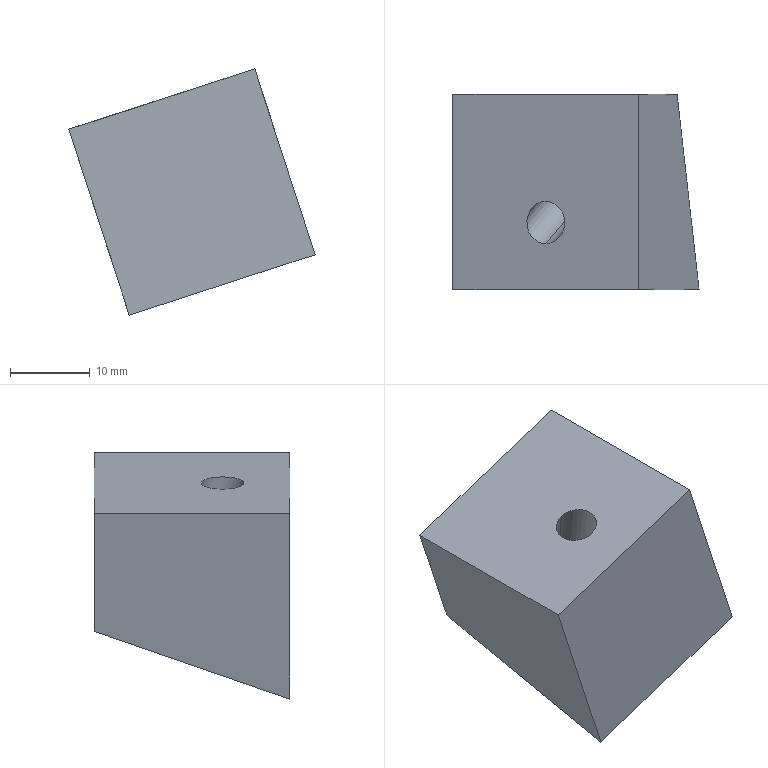Part | STEP file | 1 solid | 8 faces | box 30.872 x 24.5 x 30.872 mm | volume 11634 mm3 | plane 6 | cylinder 2 | commonest cylinder face diameters 4.998 x2
STEP:
#1=CARTESIAN_POINT('',(0.,0.,0.));
#2=DIRECTION('',(0.,0.,1.));
#3=DIRECTION('',(1.,0.,0.));
#4=AXIS2_PLACEMENT_3D('',#1,#2,#3);
#5=CARTESIAN_POINT('',(1050.233,-123.877,194.317));
#6=VERTEX_POINT('',#5);
#7=CARTESIAN_POINT('',(1050.233,-129.196,194.317));
#8=VERTEX_POINT('',#7);
#9=CARTESIAN_POINT('',(1050.233,-123.877,194.317));
#10=CARTESIAN_POINT('',(1054.986,-123.877,195.861));
#11=CARTESIAN_POINT('',(1054.986,-129.196,195.861));
#12=CARTESIAN_POINT('',(1050.233,-129.196,194.317));
#13=(BOUNDED_CURVE()B_SPLINE_CURVE(3,(#9,#10,#11,#12),.UNSPECIFIED.,.F.,.F.)B_SPLINE_CURVE_WITH_KNOTS((4,4),(0.,3.142),.PIECEWISE_BEZIER_KNOTS.)CURVE()GEOMETRIC_REPRESENTATION_ITEM()RATIONAL_B_SPLINE_CURVE((1.,0.3333,0.3333,1.))REPRESENTATION_ITEM(''));
#14=CARTESIAN_POINT('',(1061.883,-110.436,198.102));
#15=DIRECTION('',(0.309,0.,-0.9511));
#16=DIRECTION('',(0.,1.,0.));
#17=AXIS2_PLACEMENT_3D('',#14,#15,#16);
#18=PLANE('',#17);
#19=CARTESIAN_POINT('',(-13.441,-12.25));
#20=CARTESIAN_POINT('',(-13.441,-7.252));
#21=CARTESIAN_POINT('',(-18.76,-7.252));
#22=CARTESIAN_POINT('',(-18.76,-12.25));
#23=(BOUNDED_CURVE()B_SPLINE_CURVE(3,(#19,#20,#21,#22),.UNSPECIFIED.,.F.,.F.)B_SPLINE_CURVE_WITH_KNOTS((4,4),(0.,3.142),.PIECEWISE_BEZIER_KNOTS.)CURVE()GEOMETRIC_REPRESENTATION_ITEM()RATIONAL_B_SPLINE_CURVE((1.,0.3333,0.3333,1.))REPRESENTATION_ITEM(''));
#24=(GEOMETRIC_REPRESENTATION_CONTEXT(2)PARAMETRIC_REPRESENTATION_CONTEXT()REPRESENTATION_CONTEXT('',''));
#25=DEFINITIONAL_REPRESENTATION('',(#23),#24);
#26=PCURVE('',#18,#25);
#27=CARTESIAN_POINT('',(1056.084,-119.645,176.309));
#28=DIRECTION('',(0.2904,0.342,-0.8937));
#29=DIRECTION('',(-0.1057,0.9397,0.3253));
#30=AXIS2_PLACEMENT_3D('',#27,#28,#29);
#31=CYLINDRICAL_SURFACE('',#30,2.499);
#32=CARTESIAN_POINT('',(0.,-19.24));
#33=CARTESIAN_POINT('',(0.0303,-19.24));
#34=CARTESIAN_POINT('',(0.09367,-19.243));
#35=CARTESIAN_POINT('',(0.1977,-19.256));
#36=CARTESIAN_POINT('',(0.3115,-19.282));
#37=CARTESIAN_POINT('',(0.4356,-19.323));
#38=CARTESIAN_POINT('',(0.5703,-19.382));
#39=CARTESIAN_POINT('',(0.7158,-19.461));
#40=CARTESIAN_POINT('',(0.8717,-19.562));
#41=CARTESIAN_POINT('',(1.037,-19.685));
#42=CARTESIAN_POINT('',(1.21,-19.827));
#43=CARTESIAN_POINT('',(1.389,-19.984));
#44=CARTESIAN_POINT('',(1.571,-20.15));
#45=CARTESIAN_POINT('',(1.753,-20.315));
#46=CARTESIAN_POINT('',(1.931,-20.472));
#47=CARTESIAN_POINT('',(2.105,-20.615));
#48=CARTESIAN_POINT('',(2.27,-20.738));
#49=CARTESIAN_POINT('',(2.426,-20.839));
#50=CARTESIAN_POINT('',(2.571,-20.918));
#51=CARTESIAN_POINT('',(2.706,-20.977));
#52=CARTESIAN_POINT('',(2.83,-21.018));
#53=CARTESIAN_POINT('',(2.944,-21.043));
#54=CARTESIAN_POINT('',(3.048,-21.057));
#55=CARTESIAN_POINT('',(3.111,-21.059));
#56=CARTESIAN_POINT('',(3.142,-21.059));
#57=B_SPLINE_CURVE_WITH_KNOTS('',3,(#32,#33,#34,#35,#36,#37,#38,#39,#40,#41,#42,#43,#44,#45,#46,#47,#48,#49,#50,#51,#52,#53,#54,#55,#56),.UNSPECIFIED.,.F.,.F.,(4,1,1,1,1,1,1,1,1,1,1,1,1,1,1,1,1,1,1,1,1,1,4),(0.,0.1428,0.2856,0.4284,0.5712,0.714,0.8568,0.9996,1.142,1.285,1.428,1.571,1.714,1.856,1.999,2.142,2.285,2.428,2.57,2.713,2.856,2.999,3.142),.QUASI_UNIFORM_KNOTS.);
#58=(GEOMETRIC_REPRESENTATION_CONTEXT(2)PARAMETRIC_REPRESENTATION_CONTEXT()REPRESENTATION_CONTEXT('',''));
#59=DEFINITIONAL_REPRESENTATION('',(#57),#58);
#60=PCURVE('',#31,#59);
#61=SURFACE_CURVE('',#13,(#26,#60),.PCURVE_S1.);
#62=EDGE_CURVE('',#6,#8,#61,.T.);
#63=ORIENTED_EDGE('',*,*,#62,.T.);
#64=CARTESIAN_POINT('',(1050.233,-129.196,194.317));
#65=CARTESIAN_POINT('',(1045.48,-129.196,192.773));
#66=CARTESIAN_POINT('',(1045.48,-123.877,192.773));
#67=CARTESIAN_POINT('',(1050.233,-123.877,194.317));
#68=(BOUNDED_CURVE()B_SPLINE_CURVE(3,(#64,#65,#66,#67),.UNSPECIFIED.,.F.,.F.)B_SPLINE_CURVE_WITH_KNOTS((4,4),(3.142,6.283),.PIECEWISE_BEZIER_KNOTS.)CURVE()GEOMETRIC_REPRESENTATION_ITEM()RATIONAL_B_SPLINE_CURVE((1.,0.3333,0.3333,1.))REPRESENTATION_ITEM(''));
#69=CARTESIAN_POINT('',(-18.76,-12.25));
#70=CARTESIAN_POINT('',(-18.76,-17.248));
#71=CARTESIAN_POINT('',(-13.441,-17.248));
#72=CARTESIAN_POINT('',(-13.441,-12.25));
#73=(BOUNDED_CURVE()B_SPLINE_CURVE(3,(#69,#70,#71,#72),.UNSPECIFIED.,.F.,.F.)B_SPLINE_CURVE_WITH_KNOTS((4,4),(3.142,6.283),.PIECEWISE_BEZIER_KNOTS.)CURVE()GEOMETRIC_REPRESENTATION_ITEM()RATIONAL_B_SPLINE_CURVE((1.,0.3333,0.3333,1.))REPRESENTATION_ITEM(''));
#74=(GEOMETRIC_REPRESENTATION_CONTEXT(2)PARAMETRIC_REPRESENTATION_CONTEXT()REPRESENTATION_CONTEXT('',''));
#75=DEFINITIONAL_REPRESENTATION('',(#73),#74);
#76=PCURVE('',#18,#75);
#77=CARTESIAN_POINT('',(1056.084,-119.645,176.309));
#78=DIRECTION('',(0.2904,0.342,-0.8937));
#79=DIRECTION('',(-0.1057,0.9397,0.3253));
#80=AXIS2_PLACEMENT_3D('',#77,#78,#79);
#81=CYLINDRICAL_SURFACE('',#80,2.499);
#82=CARTESIAN_POINT('',(3.142,-21.059));
#83=CARTESIAN_POINT('',(3.172,-21.059));
#84=CARTESIAN_POINT('',(3.235,-21.057));
#85=CARTESIAN_POINT('',(3.339,-21.043));
#86=CARTESIAN_POINT('',(3.453,-21.018));
#87=CARTESIAN_POINT('',(3.577,-20.977));
#88=CARTESIAN_POINT('',(3.712,-20.918));
#89=CARTESIAN_POINT('',(3.857,-20.839));
#90=CARTESIAN_POINT('',(4.013,-20.738));
#91=CARTESIAN_POINT('',(4.179,-20.615));
#92=CARTESIAN_POINT('',(4.352,-20.472));
#93=CARTESIAN_POINT('',(4.531,-20.315));
#94=CARTESIAN_POINT('',(4.712,-20.15));
#95=CARTESIAN_POINT('',(4.894,-19.984));
#96=CARTESIAN_POINT('',(5.073,-19.827));
#97=CARTESIAN_POINT('',(5.246,-19.685));
#98=CARTESIAN_POINT('',(5.412,-19.562));
#99=CARTESIAN_POINT('',(5.567,-19.461));
#100=CARTESIAN_POINT('',(5.713,-19.382));
#101=CARTESIAN_POINT('',(5.848,-19.323));
#102=CARTESIAN_POINT('',(5.972,-19.282));
#103=CARTESIAN_POINT('',(6.085,-19.256));
#104=CARTESIAN_POINT('',(6.19,-19.243));
#105=CARTESIAN_POINT('',(6.253,-19.24));
#106=CARTESIAN_POINT('',(6.283,-19.24));
#107=B_SPLINE_CURVE_WITH_KNOTS('',3,(#82,#83,#84,#85,#86,#87,#88,#89,#90,#91,#92,#93,#94,#95,#96,#97,#98,#99,#100,#101,#102,#103,#104,#105,#106),.UNSPECIFIED.,.F.,.F.,(4,1,1,1,1,1,1,1,1,1,1,1,1,1,1,1,1,1,1,1,1,1,4),(3.142,3.284,3.427,3.57,3.713,3.856,3.998,4.141,4.284,4.427,4.57,4.712,4.855,4.998,5.141,5.284,5.426,5.569,5.712,5.855,5.998,6.14,6.283),.QUASI_UNIFORM_KNOTS.);
#108=(GEOMETRIC_REPRESENTATION_CONTEXT(2)PARAMETRIC_REPRESENTATION_CONTEXT()REPRESENTATION_CONTEXT('',''));
#109=DEFINITIONAL_REPRESENTATION('',(#107),#108);
#110=PCURVE('',#81,#109);
#111=SURFACE_CURVE('',#68,(#76,#110),.PCURVE_S1.);
#112=EDGE_CURVE('',#8,#6,#111,.T.);
#113=ORIENTED_EDGE('',*,*,#112,.T.);
#114=EDGE_LOOP('',(#63,#113));
#115=FACE_BOUND('',#114,.T.);
#116=CARTESIAN_POINT('',(1038.583,-134.936,190.532));
#117=VERTEX_POINT('',#116);
#118=CARTESIAN_POINT('',(1061.883,-134.936,198.102));
#119=VERTEX_POINT('',#118);
#120=CARTESIAN_POINT('',(1061.883,-134.936,198.102));
#121=DIRECTION('',(0.9511,0.,0.309));
#122=VECTOR('',#121,1.);
#123=LINE('',#120,#122);
#124=CARTESIAN_POINT('',(-24.5,0.));
#125=DIRECTION('',(0.,1.));
#126=VECTOR('',#125,1.);
#127=LINE('',#124,#126);
#128=(GEOMETRIC_REPRESENTATION_CONTEXT(2)PARAMETRIC_REPRESENTATION_CONTEXT()REPRESENTATION_CONTEXT('',''));
#129=DEFINITIONAL_REPRESENTATION('',(#127),#128);
#130=PCURVE('',#18,#129);
#131=CARTESIAN_POINT('',(1061.883,-134.936,198.102));
#132=DIRECTION('',(0.,1.,0.));
#133=DIRECTION('',(0.309,0.,-0.9511));
#134=AXIS2_PLACEMENT_3D('',#131,#132,#133);
#135=PLANE('',#134);
#136=CARTESIAN_POINT('',(0.,0.));
#137=DIRECTION('',(0.,-1.));
#138=VECTOR('',#137,1.);
#139=LINE('',#136,#138);
#140=(GEOMETRIC_REPRESENTATION_CONTEXT(2)PARAMETRIC_REPRESENTATION_CONTEXT()REPRESENTATION_CONTEXT('',''));
#141=DEFINITIONAL_REPRESENTATION('',(#139),#140);
#142=PCURVE('',#135,#141);
#143=SURFACE_CURVE('',#123,(#130,#142),.PCURVE_S1.);
#144=EDGE_CURVE('',#117,#119,#143,.T.);
#145=ORIENTED_EDGE('',*,*,#144,.T.);
#146=CARTESIAN_POINT('',(1061.883,-110.436,198.102));
#147=VERTEX_POINT('',#146);
#148=CARTESIAN_POINT('',(1061.883,-134.936,198.102));
#149=DIRECTION('',(0.,-1.,0.));
#150=VECTOR('',#149,1.);
#151=LINE('',#148,#150);
#152=CARTESIAN_POINT('',(-24.5,0.));
#153=DIRECTION('',(-1.,0.));
#154=VECTOR('',#153,1.);
#155=LINE('',#152,#154);
#156=(GEOMETRIC_REPRESENTATION_CONTEXT(2)PARAMETRIC_REPRESENTATION_CONTEXT()REPRESENTATION_CONTEXT('',''));
#157=DEFINITIONAL_REPRESENTATION('',(#155),#156);
#158=PCURVE('',#18,#157);
#159=CARTESIAN_POINT('',(1061.883,-134.936,198.102));
#160=DIRECTION('',(0.9511,0.,0.309));
#161=DIRECTION('',(0.309,0.,-0.9511));
#162=AXIS2_PLACEMENT_3D('',#159,#160,#161);
#163=PLANE('',#162);
#164=CARTESIAN_POINT('',(0.,0.));
#165=DIRECTION('',(0.,-1.));
#166=VECTOR('',#165,1.);
#167=LINE('',#164,#166);
#168=(GEOMETRIC_REPRESENTATION_CONTEXT(2)PARAMETRIC_REPRESENTATION_CONTEXT()REPRESENTATION_CONTEXT('',''));
#169=DEFINITIONAL_REPRESENTATION('',(#167),#168);
#170=PCURVE('',#163,#169);
#171=SURFACE_CURVE('',#151,(#158,#170),.PCURVE_S1.);
#172=EDGE_CURVE('',#147,#119,#171,.T.);
#173=ORIENTED_EDGE('',*,*,#172,.F.);
#174=CARTESIAN_POINT('',(1038.583,-110.436,190.532));
#175=VERTEX_POINT('',#174);
#176=CARTESIAN_POINT('',(1061.883,-110.436,198.102));
#177=DIRECTION('',(-0.9511,0.,-0.309));
#178=VECTOR('',#177,1.);
#179=LINE('',#176,#178);
#180=CARTESIAN_POINT('',(0.,0.));
#181=DIRECTION('',(0.,-1.));
#182=VECTOR('',#181,1.);
#183=LINE('',#180,#182);
#184=(GEOMETRIC_REPRESENTATION_CONTEXT(2)PARAMETRIC_REPRESENTATION_CONTEXT()REPRESENTATION_CONTEXT('',''));
#185=DEFINITIONAL_REPRESENTATION('',(#183),#184);
#186=PCURVE('',#18,#185);
#187=CARTESIAN_POINT('',(1066.699,-110.436,183.282));
#188=DIRECTION('',(0.,-1.,0.));
#189=DIRECTION('',(-0.9511,0.,-0.309));
#190=AXIS2_PLACEMENT_3D('',#187,#188,#189);
#191=PLANE('',#190);
#192=CARTESIAN_POINT('',(0.,-15.583));
#193=DIRECTION('',(1.,0.));
#194=VECTOR('',#193,1.);
#195=LINE('',#192,#194);
#196=(GEOMETRIC_REPRESENTATION_CONTEXT(2)PARAMETRIC_REPRESENTATION_CONTEXT()REPRESENTATION_CONTEXT('',''));
#197=DEFINITIONAL_REPRESENTATION('',(#195),#196);
#198=PCURVE('',#191,#197);
#199=SURFACE_CURVE('',#179,(#186,#198),.PCURVE_S1.);
#200=EDGE_CURVE('',#147,#175,#199,.T.);
#201=ORIENTED_EDGE('',*,*,#200,.T.);
#202=CARTESIAN_POINT('',(1038.583,-134.936,190.532));
#203=DIRECTION('',(0.,-1.,0.));
#204=VECTOR('',#203,1.);
#205=LINE('',#202,#204);
#206=CARTESIAN_POINT('',(-24.5,-24.5));
#207=DIRECTION('',(-1.,0.));
#208=VECTOR('',#207,1.);
#209=LINE('',#206,#208);
#210=(GEOMETRIC_REPRESENTATION_CONTEXT(2)PARAMETRIC_REPRESENTATION_CONTEXT()REPRESENTATION_CONTEXT('',''));
#211=DEFINITIONAL_REPRESENTATION('',(#209),#210);
#212=PCURVE('',#18,#211);
#213=CARTESIAN_POINT('',(1038.583,-134.936,190.532));
#214=DIRECTION('',(0.9511,0.,0.309));
#215=DIRECTION('',(0.309,0.,-0.9511));
#216=AXIS2_PLACEMENT_3D('',#213,#214,#215);
#217=PLANE('',#216);
#218=CARTESIAN_POINT('',(0.,0.));
#219=DIRECTION('',(0.,-1.));
#220=VECTOR('',#219,1.);
#221=LINE('',#218,#220);
#222=(GEOMETRIC_REPRESENTATION_CONTEXT(2)PARAMETRIC_REPRESENTATION_CONTEXT()REPRESENTATION_CONTEXT('',''));
#223=DEFINITIONAL_REPRESENTATION('',(#221),#222);
#224=PCURVE('',#217,#223);
#225=SURFACE_CURVE('',#205,(#212,#224),.PCURVE_S1.);
#226=EDGE_CURVE('',#175,#117,#225,.T.);
#227=ORIENTED_EDGE('',*,*,#226,.T.);
#228=EDGE_LOOP('',(#145,#173,#201,#227));
#229=FACE_BOUND('',#228,.T.);
#230=ADVANCED_FACE('',(#115,#229),#18,.F.);
#231=CARTESIAN_POINT('',(1046.153,-134.936,167.231));
#232=VERTEX_POINT('',#231);
#233=CARTESIAN_POINT('',(1069.454,-134.936,174.802));
#234=VERTEX_POINT('',#233);
#235=CARTESIAN_POINT('',(1069.454,-134.936,174.802));
#236=DIRECTION('',(0.9511,0.,0.309));
#237=VECTOR('',#236,1.);
#238=LINE('',#235,#237);
#239=CARTESIAN_POINT('',(24.5,0.));
#240=DIRECTION('',(0.,-1.));
#241=VECTOR('',#240,1.);
#242=LINE('',#239,#241);
#243=(GEOMETRIC_REPRESENTATION_CONTEXT(2)PARAMETRIC_REPRESENTATION_CONTEXT()REPRESENTATION_CONTEXT('',''));
#244=DEFINITIONAL_REPRESENTATION('',(#242),#243);
#245=PCURVE('',#135,#244);
#246=CARTESIAN_POINT('',(1069.454,-134.936,174.802));
#247=DIRECTION('',(-0.2904,-0.342,0.8937));
#248=DIRECTION('',(-0.1057,0.9397,0.3253));
#249=AXIS2_PLACEMENT_3D('',#246,#247,#248);
#250=PLANE('',#249);
#251=CARTESIAN_POINT('',(0.,0.));
#252=DIRECTION('',(0.,-1.));
#253=VECTOR('',#252,1.);
#254=LINE('',#251,#253);
#255=(GEOMETRIC_REPRESENTATION_CONTEXT(2)PARAMETRIC_REPRESENTATION_CONTEXT()REPRESENTATION_CONTEXT('',''));
#256=DEFINITIONAL_REPRESENTATION('',(#254),#255);
#257=PCURVE('',#250,#256);
#258=SURFACE_CURVE('',#238,(#245,#257),.PCURVE_S1.);
#259=EDGE_CURVE('',#232,#234,#258,.T.);
#260=ORIENTED_EDGE('',*,*,#259,.T.);
#261=CARTESIAN_POINT('',(1061.883,-134.936,198.102));
#262=DIRECTION('',(0.309,0.,-0.9511));
#263=VECTOR('',#262,1.);
#264=LINE('',#261,#263);
#265=CARTESIAN_POINT('',(0.,0.));
#266=DIRECTION('',(1.,0.));
#267=VECTOR('',#266,1.);
#268=LINE('',#265,#267);
#269=(GEOMETRIC_REPRESENTATION_CONTEXT(2)PARAMETRIC_REPRESENTATION_CONTEXT()REPRESENTATION_CONTEXT('',''));
#270=DEFINITIONAL_REPRESENTATION('',(#268),#269);
#271=PCURVE('',#135,#270);
#272=CARTESIAN_POINT('',(0.,0.));
#273=DIRECTION('',(1.,0.));
#274=VECTOR('',#273,1.);
#275=LINE('',#272,#274);
#276=(GEOMETRIC_REPRESENTATION_CONTEXT(2)PARAMETRIC_REPRESENTATION_CONTEXT()REPRESENTATION_CONTEXT('',''));
#277=DEFINITIONAL_REPRESENTATION('',(#275),#276);
#278=PCURVE('',#163,#277);
#279=SURFACE_CURVE('',#264,(#271,#278),.PCURVE_S1.);
#280=EDGE_CURVE('',#119,#234,#279,.T.);
#281=ORIENTED_EDGE('',*,*,#280,.F.);
#282=ORIENTED_EDGE('',*,*,#144,.F.);
#283=CARTESIAN_POINT('',(1038.583,-134.936,190.532));
#284=DIRECTION('',(0.309,0.,-0.9511));
#285=VECTOR('',#284,1.);
#286=LINE('',#283,#285);
#287=CARTESIAN_POINT('',(0.,24.5));
#288=DIRECTION('',(1.,0.));
#289=VECTOR('',#288,1.);
#290=LINE('',#287,#289);
#291=(GEOMETRIC_REPRESENTATION_CONTEXT(2)PARAMETRIC_REPRESENTATION_CONTEXT()REPRESENTATION_CONTEXT('',''));
#292=DEFINITIONAL_REPRESENTATION('',(#290),#291);
#293=PCURVE('',#135,#292);
#294=CARTESIAN_POINT('',(0.,0.));
#295=DIRECTION('',(1.,0.));
#296=VECTOR('',#295,1.);
#297=LINE('',#294,#296);
#298=(GEOMETRIC_REPRESENTATION_CONTEXT(2)PARAMETRIC_REPRESENTATION_CONTEXT()REPRESENTATION_CONTEXT('',''));
#299=DEFINITIONAL_REPRESENTATION('',(#297),#298);
#300=PCURVE('',#217,#299);
#301=SURFACE_CURVE('',#286,(#293,#300),.PCURVE_S1.);
#302=EDGE_CURVE('',#117,#232,#301,.T.);
#303=ORIENTED_EDGE('',*,*,#302,.T.);
#304=EDGE_LOOP('',(#260,#281,#282,#303));
#305=FACE_BOUND('',#304,.T.);
#306=ADVANCED_FACE('',(#305),#135,.F.);
#307=ORIENTED_EDGE('',*,*,#280,.T.);
#308=CARTESIAN_POINT('',(1066.699,-110.436,183.282));
#309=VERTEX_POINT('',#308);
#310=CARTESIAN_POINT('',(1069.454,-134.936,174.802));
#311=DIRECTION('',(-0.1057,0.9397,0.3253));
#312=VECTOR('',#311,1.);
#313=LINE('',#310,#312);
#314=CARTESIAN_POINT('',(24.5,0.));
#315=DIRECTION('',(-0.342,0.9397));
#316=VECTOR('',#315,1.);
#317=LINE('',#314,#316);
#318=(GEOMETRIC_REPRESENTATION_CONTEXT(2)PARAMETRIC_REPRESENTATION_CONTEXT()REPRESENTATION_CONTEXT('',''));
#319=DEFINITIONAL_REPRESENTATION('',(#317),#318);
#320=PCURVE('',#163,#319);
#321=CARTESIAN_POINT('',(0.,0.));
#322=DIRECTION('',(1.,0.));
#323=VECTOR('',#322,1.);
#324=LINE('',#321,#323);
#325=(GEOMETRIC_REPRESENTATION_CONTEXT(2)PARAMETRIC_REPRESENTATION_CONTEXT()REPRESENTATION_CONTEXT('',''));
#326=DEFINITIONAL_REPRESENTATION('',(#324),#325);
#327=PCURVE('',#250,#326);
#328=SURFACE_CURVE('',#313,(#320,#327),.PCURVE_S1.);
#329=EDGE_CURVE('',#234,#309,#328,.T.);
#330=ORIENTED_EDGE('',*,*,#329,.T.);
#331=CARTESIAN_POINT('',(1066.699,-110.436,183.282));
#332=DIRECTION('',(-0.309,0.,0.9511));
#333=VECTOR('',#332,1.);
#334=LINE('',#331,#333);
#335=CARTESIAN_POINT('',(15.583,24.5));
#336=DIRECTION('',(-1.,0.));
#337=VECTOR('',#336,1.);
#338=LINE('',#335,#337);
#339=(GEOMETRIC_REPRESENTATION_CONTEXT(2)PARAMETRIC_REPRESENTATION_CONTEXT()REPRESENTATION_CONTEXT('',''));
#340=DEFINITIONAL_REPRESENTATION('',(#338),#339);
#341=PCURVE('',#163,#340);
#342=CARTESIAN_POINT('',(0.,0.));
#343=DIRECTION('',(0.,-1.));
#344=VECTOR('',#343,1.);
#345=LINE('',#342,#344);
#346=(GEOMETRIC_REPRESENTATION_CONTEXT(2)PARAMETRIC_REPRESENTATION_CONTEXT()REPRESENTATION_CONTEXT('',''));
#347=DEFINITIONAL_REPRESENTATION('',(#345),#346);
#348=PCURVE('',#191,#347);
#349=SURFACE_CURVE('',#334,(#341,#348),.PCURVE_S1.);
#350=EDGE_CURVE('',#309,#147,#349,.T.);
#351=ORIENTED_EDGE('',*,*,#350,.T.);
#352=ORIENTED_EDGE('',*,*,#172,.T.);
#353=EDGE_LOOP('',(#307,#330,#351,#352));
#354=FACE_BOUND('',#353,.T.);
#355=ADVANCED_FACE('',(#354),#163,.T.);
#356=ORIENTED_EDGE('',*,*,#200,.F.);
#357=ORIENTED_EDGE('',*,*,#350,.F.);
#358=CARTESIAN_POINT('',(1043.398,-110.436,175.711));
#359=VERTEX_POINT('',#358);
#360=CARTESIAN_POINT('',(1066.699,-110.436,183.282));
#361=DIRECTION('',(-0.9511,0.,-0.309));
#362=VECTOR('',#361,1.);
#363=LINE('',#360,#362);
#364=CARTESIAN_POINT('',(0.,0.));
#365=DIRECTION('',(1.,0.));
#366=VECTOR('',#365,1.);
#367=LINE('',#364,#366);
#368=(GEOMETRIC_REPRESENTATION_CONTEXT(2)PARAMETRIC_REPRESENTATION_CONTEXT()REPRESENTATION_CONTEXT('',''));
#369=DEFINITIONAL_REPRESENTATION('',(#367),#368);
#370=PCURVE('',#191,#369);
#371=CARTESIAN_POINT('',(26.072,0.));
#372=DIRECTION('',(0.,1.));
#373=VECTOR('',#372,1.);
#374=LINE('',#371,#373);
#375=(GEOMETRIC_REPRESENTATION_CONTEXT(2)PARAMETRIC_REPRESENTATION_CONTEXT()REPRESENTATION_CONTEXT('',''));
#376=DEFINITIONAL_REPRESENTATION('',(#374),#375);
#377=PCURVE('',#250,#376);
#378=SURFACE_CURVE('',#363,(#370,#377),.PCURVE_S1.);
#379=EDGE_CURVE('',#309,#359,#378,.T.);
#380=ORIENTED_EDGE('',*,*,#379,.T.);
#381=CARTESIAN_POINT('',(1038.583,-110.436,190.532));
#382=DIRECTION('',(-0.309,0.,0.9511));
#383=VECTOR('',#382,1.);
#384=LINE('',#381,#383);
#385=CARTESIAN_POINT('',(24.5,-15.583));
#386=DIRECTION('',(0.,-1.));
#387=VECTOR('',#386,1.);
#388=LINE('',#385,#387);
#389=(GEOMETRIC_REPRESENTATION_CONTEXT(2)PARAMETRIC_REPRESENTATION_CONTEXT()REPRESENTATION_CONTEXT('',''));
#390=DEFINITIONAL_REPRESENTATION('',(#388),#389);
#391=PCURVE('',#191,#390);
#392=CARTESIAN_POINT('',(0.,24.5));
#393=DIRECTION('',(-1.,0.));
#394=VECTOR('',#393,1.);
#395=LINE('',#392,#394);
#396=(GEOMETRIC_REPRESENTATION_CONTEXT(2)PARAMETRIC_REPRESENTATION_CONTEXT()REPRESENTATION_CONTEXT('',''));
#397=DEFINITIONAL_REPRESENTATION('',(#395),#396);
#398=PCURVE('',#217,#397);
#399=SURFACE_CURVE('',#384,(#391,#398),.PCURVE_S1.);
#400=EDGE_CURVE('',#359,#175,#399,.T.);
#401=ORIENTED_EDGE('',*,*,#400,.T.);
#402=EDGE_LOOP('',(#356,#357,#380,#401));
#403=FACE_BOUND('',#402,.T.);
#404=ADVANCED_FACE('',(#403),#191,.F.);
#405=CARTESIAN_POINT('',(1046.153,-134.936,167.231));
#406=DIRECTION('',(0.1057,-0.9397,-0.3253));
#407=VECTOR('',#406,1.);
#408=LINE('',#405,#407);
#409=CARTESIAN_POINT('',(24.5,0.));
#410=DIRECTION('',(0.342,-0.9397));
#411=VECTOR('',#410,1.);
#412=LINE('',#409,#411);
#413=(GEOMETRIC_REPRESENTATION_CONTEXT(2)PARAMETRIC_REPRESENTATION_CONTEXT()REPRESENTATION_CONTEXT('',''));
#414=DEFINITIONAL_REPRESENTATION('',(#412),#413);
#415=PCURVE('',#217,#414);
#416=CARTESIAN_POINT('',(0.,24.5));
#417=DIRECTION('',(-1.,0.));
#418=VECTOR('',#417,1.);
#419=LINE('',#416,#418);
#420=(GEOMETRIC_REPRESENTATION_CONTEXT(2)PARAMETRIC_REPRESENTATION_CONTEXT()REPRESENTATION_CONTEXT('',''));
#421=DEFINITIONAL_REPRESENTATION('',(#419),#420);
#422=PCURVE('',#250,#421);
#423=SURFACE_CURVE('',#408,(#415,#422),.PCURVE_S1.);
#424=EDGE_CURVE('',#359,#232,#423,.T.);
#425=ORIENTED_EDGE('',*,*,#424,.T.);
#426=ORIENTED_EDGE('',*,*,#302,.F.);
#427=ORIENTED_EDGE('',*,*,#226,.F.);
#428=ORIENTED_EDGE('',*,*,#400,.F.);
#429=EDGE_LOOP('',(#425,#426,#427,#428));
#430=FACE_BOUND('',#429,.T.);
#431=ADVANCED_FACE('',(#430),#217,.F.);
#432=CARTESIAN_POINT('',(1055.82,-117.297,177.122));
#433=VERTEX_POINT('',#432);
#434=CARTESIAN_POINT('',(1056.348,-121.993,175.496));
#435=VERTEX_POINT('',#434);
#436=CARTESIAN_POINT('',(1056.084,-119.645,176.309));
#437=DIRECTION('',(0.2904,0.342,-0.8937));
#438=DIRECTION('',(-0.1057,0.9397,0.3253));
#439=AXIS2_PLACEMENT_3D('',#436,#437,#438);
#440=CIRCLE('',#439,2.499);
#441=CARTESIAN_POINT('',(0.,0.));
#442=DIRECTION('',(1.,0.));
#443=VECTOR('',#442,1.);
#444=LINE('',#441,#443);
#445=(GEOMETRIC_REPRESENTATION_CONTEXT(2)PARAMETRIC_REPRESENTATION_CONTEXT()REPRESENTATION_CONTEXT('',''));
#446=DEFINITIONAL_REPRESENTATION('',(#444),#445);
#447=PCURVE('',#31,#446);
#448=CARTESIAN_POINT('',(18.771,12.25));
#449=CARTESIAN_POINT('',(18.771,7.922));
#450=CARTESIAN_POINT('',(15.023,10.086));
#451=CARTESIAN_POINT('',(11.274,12.25));
#452=CARTESIAN_POINT('',(15.023,14.414));
#453=CARTESIAN_POINT('',(18.771,16.578));
#454=CARTESIAN_POINT('',(18.771,12.25));
#455=(BOUNDED_CURVE()B_SPLINE_CURVE(2,(#448,#449,#450,#451,#452,#453,#454),.UNSPECIFIED.,.T.,.F.)B_SPLINE_CURVE_WITH_KNOTS((1,2,2,2,2,1),(-2.094,0.,2.094,4.189,6.283,8.378),.UNSPECIFIED.)CURVE()GEOMETRIC_REPRESENTATION_ITEM()RATIONAL_B_SPLINE_CURVE((1.,0.5,1.,0.5,1.,0.5,1.))REPRESENTATION_ITEM(''));
#456=(GEOMETRIC_REPRESENTATION_CONTEXT(2)PARAMETRIC_REPRESENTATION_CONTEXT()REPRESENTATION_CONTEXT('',''));
#457=DEFINITIONAL_REPRESENTATION('',(#455),#456);
#458=PCURVE('',#250,#457);
#459=SURFACE_CURVE('',#440,(#447,#458),.PCURVE_S1.);
#460=EDGE_CURVE('',#433,#435,#459,.T.);
#461=ORIENTED_EDGE('',*,*,#460,.F.);
#462=CARTESIAN_POINT('',(1055.82,-117.297,177.122));
#463=DIRECTION('',(0.2904,0.342,-0.8937));
#464=VECTOR('',#463,1.);
#465=LINE('',#462,#464);
#466=CARTESIAN_POINT('',(0.,0.));
#467=DIRECTION('',(0.,1.));
#468=VECTOR('',#467,1.);
#469=LINE('',#466,#468);
#470=(GEOMETRIC_REPRESENTATION_CONTEXT(2)PARAMETRIC_REPRESENTATION_CONTEXT()REPRESENTATION_CONTEXT('',''));
#471=DEFINITIONAL_REPRESENTATION('',(#469),#470);
#472=PCURVE('',#31,#471);
#473=CARTESIAN_POINT('',(6.283,0.));
#474=DIRECTION('',(0.,1.));
#475=VECTOR('',#474,1.);
#476=LINE('',#473,#475);
#477=(GEOMETRIC_REPRESENTATION_CONTEXT(2)PARAMETRIC_REPRESENTATION_CONTEXT()REPRESENTATION_CONTEXT('',''));
#478=DEFINITIONAL_REPRESENTATION('',(#476),#477);
#479=PCURVE('',#81,#478);
#480=SURFACE_CURVE('',#465,(#472,#479),.PCURVE_S1.);
#481=EDGE_CURVE('',#6,#433,#480,.T.);
#482=ORIENTED_EDGE('',*,*,#481,.F.);
#483=ORIENTED_EDGE('',*,*,#62,.T.);
#484=CARTESIAN_POINT('',(1056.348,-121.993,175.496));
#485=DIRECTION('',(0.2904,0.342,-0.8937));
#486=VECTOR('',#485,1.);
#487=LINE('',#484,#486);
#488=CARTESIAN_POINT('',(3.142,0.));
#489=DIRECTION('',(0.,1.));
#490=VECTOR('',#489,1.);
#491=LINE('',#488,#490);
#492=(GEOMETRIC_REPRESENTATION_CONTEXT(2)PARAMETRIC_REPRESENTATION_CONTEXT()REPRESENTATION_CONTEXT('',''));
#493=DEFINITIONAL_REPRESENTATION('',(#491),#492);
#494=PCURVE('',#31,#493);
#495=CARTESIAN_POINT('',(3.142,0.));
#496=DIRECTION('',(0.,1.));
#497=VECTOR('',#496,1.);
#498=LINE('',#495,#497);
#499=(GEOMETRIC_REPRESENTATION_CONTEXT(2)PARAMETRIC_REPRESENTATION_CONTEXT()REPRESENTATION_CONTEXT('',''));
#500=DEFINITIONAL_REPRESENTATION('',(#498),#499);
#501=PCURVE('',#81,#500);
#502=SURFACE_CURVE('',#487,(#494,#501),.PCURVE_S1.);
#503=EDGE_CURVE('',#8,#435,#502,.T.);
#504=ORIENTED_EDGE('',*,*,#503,.T.);
#505=EDGE_LOOP('',(#461,#482,#483,#504));
#506=FACE_BOUND('',#505,.F.);
#507=ADVANCED_FACE('',(#506),#31,.F.);
#508=ORIENTED_EDGE('',*,*,#460,.F.);
#509=CARTESIAN_POINT('',(1056.084,-119.645,176.309));
#510=DIRECTION('',(0.2904,0.342,-0.8937));
#511=DIRECTION('',(-0.1057,0.9397,0.3253));
#512=AXIS2_PLACEMENT_3D('',#509,#510,#511);
#513=CIRCLE('',#512,2.499);
#514=CARTESIAN_POINT('',(18.771,12.25));
#515=CARTESIAN_POINT('',(18.771,7.922));
#516=CARTESIAN_POINT('',(15.023,10.086));
#517=CARTESIAN_POINT('',(11.274,12.25));
#518=CARTESIAN_POINT('',(15.023,14.414));
#519=CARTESIAN_POINT('',(18.771,16.578));
#520=CARTESIAN_POINT('',(18.771,12.25));
#521=(BOUNDED_CURVE()B_SPLINE_CURVE(2,(#514,#515,#516,#517,#518,#519,#520),.UNSPECIFIED.,.T.,.F.)B_SPLINE_CURVE_WITH_KNOTS((1,2,2,2,2,1),(-2.094,0.,2.094,4.189,6.283,8.378),.UNSPECIFIED.)CURVE()GEOMETRIC_REPRESENTATION_ITEM()RATIONAL_B_SPLINE_CURVE((1.,0.5,1.,0.5,1.,0.5,1.))REPRESENTATION_ITEM(''));
#522=(GEOMETRIC_REPRESENTATION_CONTEXT(2)PARAMETRIC_REPRESENTATION_CONTEXT()REPRESENTATION_CONTEXT('',''));
#523=DEFINITIONAL_REPRESENTATION('',(#521),#522);
#524=PCURVE('',#250,#523);
#525=CARTESIAN_POINT('',(0.,0.));
#526=DIRECTION('',(1.,0.));
#527=VECTOR('',#526,1.);
#528=LINE('',#525,#527);
#529=(GEOMETRIC_REPRESENTATION_CONTEXT(2)PARAMETRIC_REPRESENTATION_CONTEXT()REPRESENTATION_CONTEXT('',''));
#530=DEFINITIONAL_REPRESENTATION('',(#528),#529);
#531=PCURVE('',#81,#530);
#532=SURFACE_CURVE('',#513,(#524,#531),.PCURVE_S1.);
#533=EDGE_CURVE('',#435,#433,#532,.T.);
#534=ORIENTED_EDGE('',*,*,#533,.F.);
#535=EDGE_LOOP('',(#508,#534));
#536=FACE_BOUND('',#535,.T.);
#537=ORIENTED_EDGE('',*,*,#379,.F.);
#538=ORIENTED_EDGE('',*,*,#329,.F.);
#539=ORIENTED_EDGE('',*,*,#259,.F.);
#540=ORIENTED_EDGE('',*,*,#424,.F.);
#541=EDGE_LOOP('',(#537,#538,#539,#540));
#542=FACE_BOUND('',#541,.T.);
#543=ADVANCED_FACE('',(#536,#542),#250,.F.);
#544=ORIENTED_EDGE('',*,*,#481,.T.);
#545=ORIENTED_EDGE('',*,*,#533,.F.);
#546=ORIENTED_EDGE('',*,*,#503,.F.);
#547=ORIENTED_EDGE('',*,*,#112,.T.);
#548=EDGE_LOOP('',(#544,#545,#546,#547));
#549=FACE_BOUND('',#548,.F.);
#550=ADVANCED_FACE('',(#549),#81,.F.);
#551=CLOSED_SHELL('',(#230,#306,#355,#404,#431,#507,#543,#550));
#552=MANIFOLD_SOLID_BREP('',#551);
#553=(LENGTH_UNIT()NAMED_UNIT(*)SI_UNIT(.MILLI.,.METRE.));
#554=UNCERTAINTY_MEASURE_WITH_UNIT(LENGTH_MEASURE(0.0000001),#553,'','');
#555=(NAMED_UNIT(*)PLANE_ANGLE_UNIT()SI_UNIT($,.RADIAN.));
#556=(NAMED_UNIT(*)SI_UNIT($,.STERADIAN.)SOLID_ANGLE_UNIT());
#557=(GEOMETRIC_REPRESENTATION_CONTEXT(3)GLOBAL_UNCERTAINTY_ASSIGNED_CONTEXT((#554))GLOBAL_UNIT_ASSIGNED_CONTEXT((#553,#555,#556))REPRESENTATION_CONTEXT('',''));
#558=ADVANCED_BREP_SHAPE_REPRESENTATION('',(#4,#552),#557);